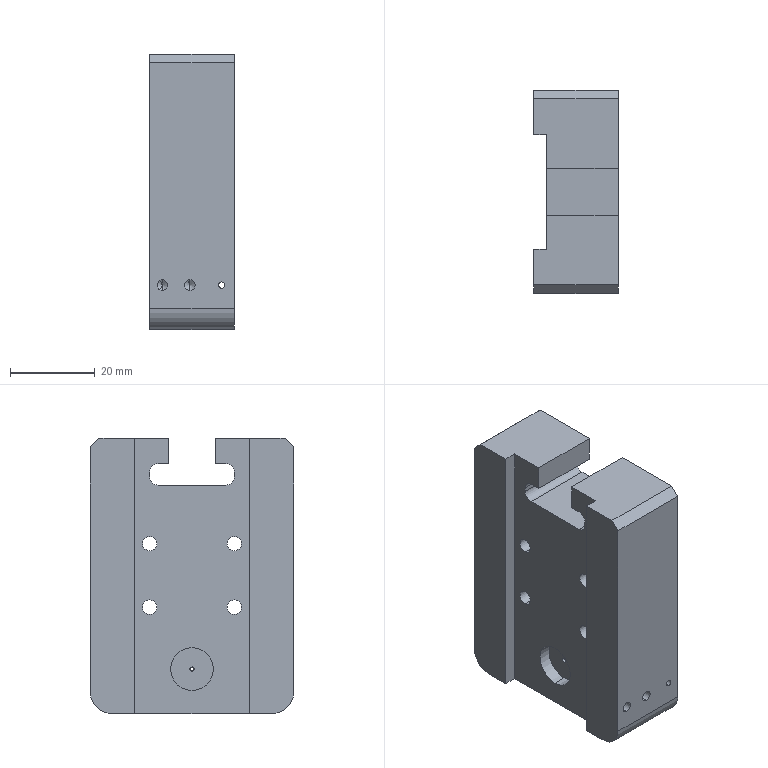Part | SolidWorks | features ICE 6, HoleWzd 3, Chamfer 2, Fillet 2, Extrusion 1, MoveFace 1 | 1 solid | 84 faces | box 20 x 48 x 65 mm | volume 52425 mm3 | cylinder 44 | plane 26 | cone 14 | commonest cylinder face diameters 2.5 x12 3.4 x8 6 x8 1.5 x4 4 x4 1 x2